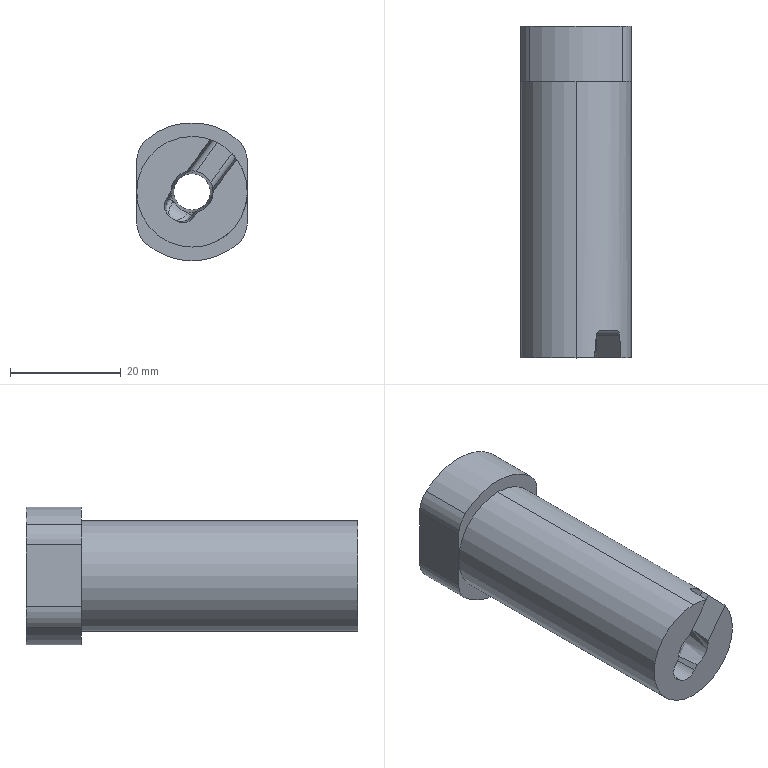Part | STEP file | 1 solid | 34 faces | box 20 x 60 x 25 mm | volume 17460 mm3 | cylinder 16 | plane 14 | cone 2 | spline 2 | commonest cylinder face diameters 2 x4 10 x4 5 x3 25 x3 20 x2